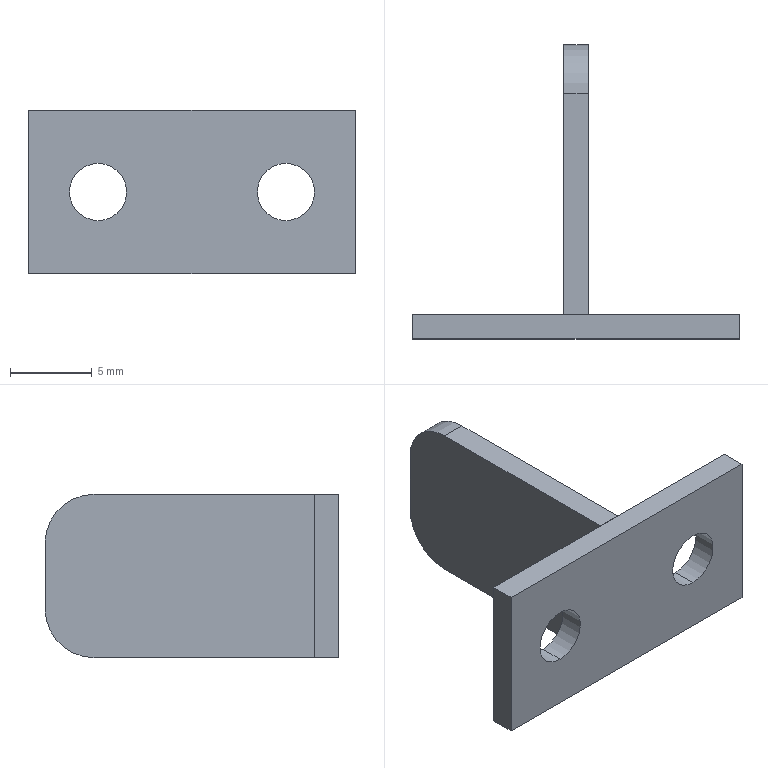Part | STEP file | Sensor detection tab | 2 solids | 18 faces | box 20 x 18 x 10 mm | volume 512.842 mm3 | plane 12 | cylinder 6 | commonest cylinder face diameters 3.5 x4 6 x2
STEP:
#1=CARTESIAN_POINT('',(0.75,13.5,-5.));
#2=VERTEX_POINT('',#1);
#3=CARTESIAN_POINT('',(0.75,0.,-5.));
#4=VERTEX_POINT('',#3);
#5=CARTESIAN_POINT('',(0.75,16.5,-5.));
#6=DIRECTION('',(0.,-1.,0.));
#7=VECTOR('',#6,1000.);
#8=LINE('',#5,#7);
#9=EDGE_CURVE('',#2,#4,#8,.T.);
#10=ORIENTED_EDGE('',*,*,#9,.F.);
#11=CARTESIAN_POINT('',(0.75,16.5,-2.));
#12=VERTEX_POINT('',#11);
#13=CARTESIAN_POINT('',(0.75,13.5,-2.));
#14=DIRECTION('',(1.,0.,0.));
#15=DIRECTION('',(0.,0.,1.));
#16=AXIS2_PLACEMENT_3D('',#13,#14,#15);
#17=CIRCLE('',#16,3.);
#18=EDGE_CURVE('',#2,#12,#17,.T.);
#19=ORIENTED_EDGE('',*,*,#18,.T.);
#20=CARTESIAN_POINT('',(0.75,16.5,2.));
#21=VERTEX_POINT('',#20);
#22=CARTESIAN_POINT('',(0.75,16.5,-5.));
#23=DIRECTION('',(0.,0.,-1.));
#24=VECTOR('',#23,1000.);
#25=LINE('',#22,#24);
#26=EDGE_CURVE('',#21,#12,#25,.T.);
#27=ORIENTED_EDGE('',*,*,#26,.F.);
#28=CARTESIAN_POINT('',(0.75,13.5,5.));
#29=VERTEX_POINT('',#28);
#30=CARTESIAN_POINT('',(0.75,13.5,2.));
#31=DIRECTION('',(1.,0.,0.));
#32=DIRECTION('',(0.,0.,1.));
#33=AXIS2_PLACEMENT_3D('',#30,#31,#32);
#34=CIRCLE('',#33,3.);
#35=EDGE_CURVE('',#21,#29,#34,.T.);
#36=ORIENTED_EDGE('',*,*,#35,.T.);
#37=CARTESIAN_POINT('',(0.75,0.,5.));
#38=VERTEX_POINT('',#37);
#39=CARTESIAN_POINT('',(0.75,16.5,5.));
#40=DIRECTION('',(0.,-1.,0.));
#41=VECTOR('',#40,1000.);
#42=LINE('',#39,#41);
#43=EDGE_CURVE('',#29,#38,#42,.T.);
#44=ORIENTED_EDGE('',*,*,#43,.T.);
#45=CARTESIAN_POINT('',(0.75,0.,-5.));
#46=DIRECTION('',(0.,0.,-1.));
#47=VECTOR('',#46,1000.);
#48=LINE('',#45,#47);
#49=EDGE_CURVE('',#38,#4,#48,.T.);
#50=ORIENTED_EDGE('',*,*,#49,.T.);
#51=EDGE_LOOP('',(#10,#19,#27,#36,#44,#50));
#52=FACE_OUTER_BOUND('',#51,.T.);
#53=CARTESIAN_POINT('',(0.75,16.5,-5.));
#54=DIRECTION('',(-1.,0.,0.));
#55=DIRECTION('',(0.,0.,1.));
#56=AXIS2_PLACEMENT_3D('',#53,#54,#55);
#57=PLANE('',#56);
#58=ADVANCED_FACE('',(#52),#57,.F.);
#59=CARTESIAN_POINT('',(-0.75,13.5,-5.));
#60=VERTEX_POINT('',#59);
#61=CARTESIAN_POINT('',(-0.75,0.,-5.));
#62=VERTEX_POINT('',#61);
#63=CARTESIAN_POINT('',(-0.75,16.5,-5.));
#64=DIRECTION('',(0.,-1.,0.));
#65=VECTOR('',#64,1000.);
#66=LINE('',#63,#65);
#67=EDGE_CURVE('',#60,#62,#66,.T.);
#68=ORIENTED_EDGE('',*,*,#67,.F.);
#69=CARTESIAN_POINT('',(0.75,13.5,-5.));
#70=DIRECTION('',(1.,0.,0.));
#71=VECTOR('',#70,1000.);
#72=LINE('',#69,#71);
#73=EDGE_CURVE('',#60,#2,#72,.T.);
#74=ORIENTED_EDGE('',*,*,#73,.T.);
#75=ORIENTED_EDGE('',*,*,#9,.T.);
#76=CARTESIAN_POINT('',(-0.75,0.,-5.));
#77=DIRECTION('',(-1.,0.,0.));
#78=VECTOR('',#77,1000.);
#79=LINE('',#76,#78);
#80=EDGE_CURVE('',#4,#62,#79,.T.);
#81=ORIENTED_EDGE('',*,*,#80,.T.);
#82=EDGE_LOOP('',(#68,#74,#75,#81));
#83=FACE_OUTER_BOUND('',#82,.T.);
#84=CARTESIAN_POINT('',(-0.75,16.5,-5.));
#85=DIRECTION('',(0.,0.,1.));
#86=DIRECTION('',(1.,0.,0.));
#87=AXIS2_PLACEMENT_3D('',#84,#85,#86);
#88=PLANE('',#87);
#89=ADVANCED_FACE('',(#83),#88,.F.);
#90=CARTESIAN_POINT('',(-0.75,16.5,-2.));
#91=VERTEX_POINT('',#90);
#92=CARTESIAN_POINT('',(-0.75,16.5,2.));
#93=VERTEX_POINT('',#92);
#94=CARTESIAN_POINT('',(-0.75,16.5,-5.));
#95=DIRECTION('',(0.,0.,1.));
#96=VECTOR('',#95,1000.);
#97=LINE('',#94,#96);
#98=EDGE_CURVE('',#91,#93,#97,.T.);
#99=ORIENTED_EDGE('',*,*,#98,.F.);
#100=CARTESIAN_POINT('',(-0.75,13.5,-2.));
#101=DIRECTION('',(-1.,0.,0.));
#102=DIRECTION('',(0.,0.,-1.));
#103=AXIS2_PLACEMENT_3D('',#100,#101,#102);
#104=CIRCLE('',#103,3.);
#105=EDGE_CURVE('',#91,#60,#104,.T.);
#106=ORIENTED_EDGE('',*,*,#105,.T.);
#107=ORIENTED_EDGE('',*,*,#67,.T.);
#108=CARTESIAN_POINT('',(-0.75,0.,5.));
#109=VERTEX_POINT('',#108);
#110=CARTESIAN_POINT('',(-0.75,0.,-5.));
#111=DIRECTION('',(0.,0.,1.));
#112=VECTOR('',#111,1000.);
#113=LINE('',#110,#112);
#114=EDGE_CURVE('',#62,#109,#113,.T.);
#115=ORIENTED_EDGE('',*,*,#114,.T.);
#116=CARTESIAN_POINT('',(-0.75,13.5,5.));
#117=VERTEX_POINT('',#116);
#118=CARTESIAN_POINT('',(-0.75,16.5,5.));
#119=DIRECTION('',(0.,-1.,0.));
#120=VECTOR('',#119,1000.);
#121=LINE('',#118,#120);
#122=EDGE_CURVE('',#117,#109,#121,.T.);
#123=ORIENTED_EDGE('',*,*,#122,.F.);
#124=CARTESIAN_POINT('',(-0.75,13.5,2.));
#125=DIRECTION('',(-1.,0.,0.));
#126=DIRECTION('',(0.,0.,-1.));
#127=AXIS2_PLACEMENT_3D('',#124,#125,#126);
#128=CIRCLE('',#127,3.);
#129=EDGE_CURVE('',#117,#93,#128,.T.);
#130=ORIENTED_EDGE('',*,*,#129,.T.);
#131=EDGE_LOOP('',(#99,#106,#107,#115,#123,#130));
#132=FACE_OUTER_BOUND('',#131,.T.);
#133=CARTESIAN_POINT('',(-0.75,16.5,-5.));
#134=DIRECTION('',(1.,0.,0.));
#135=DIRECTION('',(0.,0.,-1.));
#136=AXIS2_PLACEMENT_3D('',#133,#134,#135);
#137=PLANE('',#136);
#138=ADVANCED_FACE('',(#132),#137,.F.);
#139=ORIENTED_EDGE('',*,*,#43,.F.);
#140=CARTESIAN_POINT('',(-0.75,13.5,5.));
#141=DIRECTION('',(-1.,0.,0.));
#142=VECTOR('',#141,1000.);
#143=LINE('',#140,#142);
#144=EDGE_CURVE('',#29,#117,#143,.T.);
#145=ORIENTED_EDGE('',*,*,#144,.T.);
#146=ORIENTED_EDGE('',*,*,#122,.T.);
#147=CARTESIAN_POINT('',(-0.75,0.,5.));
#148=DIRECTION('',(1.,0.,0.));
#149=VECTOR('',#148,1000.);
#150=LINE('',#147,#149);
#151=EDGE_CURVE('',#109,#38,#150,.T.);
#152=ORIENTED_EDGE('',*,*,#151,.T.);
#153=EDGE_LOOP('',(#139,#145,#146,#152));
#154=FACE_OUTER_BOUND('',#153,.T.);
#155=CARTESIAN_POINT('',(-0.75,16.5,5.));
#156=DIRECTION('',(0.,0.,-1.));
#157=DIRECTION('',(-1.,0.,0.));
#158=AXIS2_PLACEMENT_3D('',#155,#156,#157);
#159=PLANE('',#158);
#160=ADVANCED_FACE('',(#154),#159,.F.);
#161=ORIENTED_EDGE('',*,*,#26,.T.);
#162=CARTESIAN_POINT('',(-0.75,16.5,-2.));
#163=DIRECTION('',(-1.,0.,0.));
#164=VECTOR('',#163,1000.);
#165=LINE('',#162,#164);
#166=EDGE_CURVE('',#12,#91,#165,.T.);
#167=ORIENTED_EDGE('',*,*,#166,.T.);
#168=ORIENTED_EDGE('',*,*,#98,.T.);
#169=CARTESIAN_POINT('',(0.75,16.5,2.));
#170=DIRECTION('',(1.,0.,0.));
#171=VECTOR('',#170,1000.);
#172=LINE('',#169,#171);
#173=EDGE_CURVE('',#93,#21,#172,.T.);
#174=ORIENTED_EDGE('',*,*,#173,.T.);
#175=EDGE_LOOP('',(#161,#167,#168,#174));
#176=FACE_OUTER_BOUND('',#175,.T.);
#177=CARTESIAN_POINT('',(0.,16.5,0.));
#178=DIRECTION('',(0.,1.,0.));
#179=DIRECTION('',(0.,0.,1.));
#180=AXIS2_PLACEMENT_3D('',#177,#178,#179);
#181=PLANE('',#180);
#182=ADVANCED_FACE('',(#176),#181,.T.);
#183=ORIENTED_EDGE('',*,*,#49,.F.);
#184=ORIENTED_EDGE('',*,*,#151,.F.);
#185=ORIENTED_EDGE('',*,*,#114,.F.);
#186=ORIENTED_EDGE('',*,*,#80,.F.);
#187=EDGE_LOOP('',(#183,#184,#185,#186));
#188=FACE_OUTER_BOUND('',#187,.T.);
#189=CARTESIAN_POINT('',(0.,0.,0.));
#190=DIRECTION('',(0.,1.,0.));
#191=DIRECTION('',(0.,0.,1.));
#192=AXIS2_PLACEMENT_3D('',#189,#190,#191);
#193=PLANE('',#192);
#194=ADVANCED_FACE('',(#188),#193,.F.);
#195=ORIENTED_EDGE('',*,*,#18,.F.);
#196=ORIENTED_EDGE('',*,*,#73,.F.);
#197=ORIENTED_EDGE('',*,*,#105,.F.);
#198=ORIENTED_EDGE('',*,*,#166,.F.);
#199=EDGE_LOOP('',(#195,#196,#197,#198));
#200=FACE_OUTER_BOUND('',#199,.T.);
#201=CARTESIAN_POINT('',(0.,13.5,-2.));
#202=DIRECTION('',(1.,0.,0.));
#203=DIRECTION('',(0.,0.,-1.));
#204=AXIS2_PLACEMENT_3D('',#201,#202,#203);
#205=CYLINDRICAL_SURFACE('',#204,3.);
#206=ADVANCED_FACE('',(#200),#205,.T.);
#207=ORIENTED_EDGE('',*,*,#129,.F.);
#208=ORIENTED_EDGE('',*,*,#144,.F.);
#209=ORIENTED_EDGE('',*,*,#35,.F.);
#210=ORIENTED_EDGE('',*,*,#173,.F.);
#211=EDGE_LOOP('',(#207,#208,#209,#210));
#212=FACE_OUTER_BOUND('',#211,.T.);
#213=CARTESIAN_POINT('',(0.,13.5,2.));
#214=DIRECTION('',(-1.,0.,0.));
#215=DIRECTION('',(0.,0.,1.));
#216=AXIS2_PLACEMENT_3D('',#213,#214,#215);
#217=CYLINDRICAL_SURFACE('',#216,3.);
#218=ADVANCED_FACE('',(#212),#217,.T.);
#219=CLOSED_SHELL('',(#58,#89,#138,#160,#182,#194,#206,#218));
#220=MANIFOLD_SOLID_BREP('',#219);
#221=CARTESIAN_POINT('',(-5.75,-1.5,-1.75));
#222=VERTEX_POINT('',#221);
#223=CARTESIAN_POINT('',(-5.75,-1.5,1.75));
#224=VERTEX_POINT('',#223);
#225=CARTESIAN_POINT('',(-5.75,-1.5,0.));
#226=DIRECTION('',(0.,1.,0.));
#227=DIRECTION('',(0.,0.,1.));
#228=AXIS2_PLACEMENT_3D('',#225,#226,#227);
#229=CIRCLE('',#228,1.75);
#230=EDGE_CURVE('',#222,#224,#229,.T.);
#231=ORIENTED_EDGE('',*,*,#230,.F.);
#232=CARTESIAN_POINT('',(-5.75,0.,-1.75));
#233=VERTEX_POINT('',#232);
#234=CARTESIAN_POINT('',(-5.75,0.,-1.75));
#235=DIRECTION('',(0.,1.,0.));
#236=VECTOR('',#235,1000.);
#237=LINE('',#234,#236);
#238=EDGE_CURVE('',#222,#233,#237,.T.);
#239=ORIENTED_EDGE('',*,*,#238,.T.);
#240=CARTESIAN_POINT('',(-5.75,0.,1.75));
#241=VERTEX_POINT('',#240);
#242=CARTESIAN_POINT('',(-5.75,0.,0.));
#243=DIRECTION('',(0.,1.,0.));
#244=DIRECTION('',(0.,0.,1.));
#245=AXIS2_PLACEMENT_3D('',#242,#243,#244);
#246=CIRCLE('',#245,1.75);
#247=EDGE_CURVE('',#233,#241,#246,.T.);
#248=ORIENTED_EDGE('',*,*,#247,.T.);
#249=CARTESIAN_POINT('',(-5.75,0.,1.75));
#250=DIRECTION('',(0.,1.,0.));
#251=VECTOR('',#250,1000.);
#252=LINE('',#249,#251);
#253=EDGE_CURVE('',#224,#241,#252,.T.);
#254=ORIENTED_EDGE('',*,*,#253,.F.);
#255=EDGE_LOOP('',(#231,#239,#248,#254));
#256=FACE_OUTER_BOUND('',#255,.T.);
#257=CARTESIAN_POINT('',(-5.75,0.,0.));
#258=DIRECTION('',(0.,1.,0.));
#259=DIRECTION('',(0.,0.,1.));
#260=AXIS2_PLACEMENT_3D('',#257,#258,#259);
#261=CYLINDRICAL_SURFACE('',#260,1.75);
#262=ADVANCED_FACE('',(#256),#261,.F.);
#263=CARTESIAN_POINT('',(5.75,-1.5,-1.75));
#264=VERTEX_POINT('',#263);
#265=CARTESIAN_POINT('',(5.75,-1.5,1.75));
#266=VERTEX_POINT('',#265);
#267=CARTESIAN_POINT('',(5.75,-1.5,0.));
#268=DIRECTION('',(0.,1.,0.));
#269=DIRECTION('',(0.,0.,1.));
#270=AXIS2_PLACEMENT_3D('',#267,#268,#269);
#271=CIRCLE('',#270,1.75);
#272=EDGE_CURVE('',#264,#266,#271,.T.);
#273=ORIENTED_EDGE('',*,*,#272,.F.);
#274=CARTESIAN_POINT('',(5.75,0.,-1.75));
#275=VERTEX_POINT('',#274);
#276=CARTESIAN_POINT('',(5.75,0.,-1.75));
#277=DIRECTION('',(0.,1.,0.));
#278=VECTOR('',#277,1000.);
#279=LINE('',#276,#278);
#280=EDGE_CURVE('',#264,#275,#279,.T.);
#281=ORIENTED_EDGE('',*,*,#280,.T.);
#282=CARTESIAN_POINT('',(5.75,0.,1.75));
#283=VERTEX_POINT('',#282);
#284=CARTESIAN_POINT('',(5.75,0.,0.));
#285=DIRECTION('',(0.,1.,0.));
#286=DIRECTION('',(0.,0.,1.));
#287=AXIS2_PLACEMENT_3D('',#284,#285,#286);
#288=CIRCLE('',#287,1.75);
#289=EDGE_CURVE('',#275,#283,#288,.T.);
#290=ORIENTED_EDGE('',*,*,#289,.T.);
#291=CARTESIAN_POINT('',(5.75,0.,1.75));
#292=DIRECTION('',(0.,1.,0.));
#293=VECTOR('',#292,1000.);
#294=LINE('',#291,#293);
#295=EDGE_CURVE('',#266,#283,#294,.T.);
#296=ORIENTED_EDGE('',*,*,#295,.F.);
#297=EDGE_LOOP('',(#273,#281,#290,#296));
#298=FACE_OUTER_BOUND('',#297,.T.);
#299=CARTESIAN_POINT('',(5.75,0.,0.));
#300=DIRECTION('',(0.,1.,0.));
#301=DIRECTION('',(0.,0.,1.));
#302=AXIS2_PLACEMENT_3D('',#299,#300,#301);
#303=CYLINDRICAL_SURFACE('',#302,1.75);
#304=ADVANCED_FACE('',(#298),#303,.F.);
#305=CARTESIAN_POINT('',(10.,0.,5.));
#306=VERTEX_POINT('',#305);
#307=CARTESIAN_POINT('',(10.,0.,-5.));
#308=VERTEX_POINT('',#307);
#309=CARTESIAN_POINT('',(10.,0.,-5.));
#310=DIRECTION('',(0.,0.,-1.));
#311=VECTOR('',#310,1000.);
#312=LINE('',#309,#311);
#313=EDGE_CURVE('',#306,#308,#312,.T.);
#314=ORIENTED_EDGE('',*,*,#313,.F.);
#315=CARTESIAN_POINT('',(10.,-1.5,5.));
#316=VERTEX_POINT('',#315);
#317=CARTESIAN_POINT('',(10.,-1.5,5.));
#318=DIRECTION('',(0.,1.,0.));
#319=VECTOR('',#318,1000.);
#320=LINE('',#317,#319);
#321=EDGE_CURVE('',#316,#306,#320,.T.);
#322=ORIENTED_EDGE('',*,*,#321,.F.);
#323=CARTESIAN_POINT('',(10.,-1.5,-5.));
#324=VERTEX_POINT('',#323);
#325=CARTESIAN_POINT('',(10.,-1.5,-5.));
#326=DIRECTION('',(0.,0.,-1.));
#327=VECTOR('',#326,1000.);
#328=LINE('',#325,#327);
#329=EDGE_CURVE('',#316,#324,#328,.T.);
#330=ORIENTED_EDGE('',*,*,#329,.T.);
#331=CARTESIAN_POINT('',(10.,-1.5,-5.));
#332=DIRECTION('',(0.,1.,0.));
#333=VECTOR('',#332,1000.);
#334=LINE('',#331,#333);
#335=EDGE_CURVE('',#324,#308,#334,.T.);
#336=ORIENTED_EDGE('',*,*,#335,.T.);
#337=EDGE_LOOP('',(#314,#322,#330,#336));
#338=FACE_OUTER_BOUND('',#337,.T.);
#339=CARTESIAN_POINT('',(10.,-1.5,-5.));
#340=DIRECTION('',(1.,0.,0.));
#341=DIRECTION('',(0.,0.,-1.));
#342=AXIS2_PLACEMENT_3D('',#339,#340,#341);
#343=PLANE('',#342);
#344=ADVANCED_FACE('',(#338),#343,.T.);
#345=CARTESIAN_POINT('',(-10.,0.,5.));
#346=VERTEX_POINT('',#345);
#347=CARTESIAN_POINT('',(-10.,0.,5.));
#348=DIRECTION('',(1.,0.,0.));
#349=VECTOR('',#348,1000.);
#350=LINE('',#347,#349);
#351=EDGE_CURVE('',#346,#306,#350,.T.);
#352=ORIENTED_EDGE('',*,*,#351,.F.);
#353=CARTESIAN_POINT('',(-10.,-1.5,5.));
#354=VERTEX_POINT('',#353);
#355=CARTESIAN_POINT('',(-10.,-1.5,5.));
#356=DIRECTION('',(0.,1.,0.));
#357=VECTOR('',#356,1000.);
#358=LINE('',#355,#357);
#359=EDGE_CURVE('',#354,#346,#358,.T.);
#360=ORIENTED_EDGE('',*,*,#359,.F.);
#361=CARTESIAN_POINT('',(-10.,-1.5,5.));
#362=DIRECTION('',(1.,0.,0.));
#363=VECTOR('',#362,1000.);
#364=LINE('',#361,#363);
#365=EDGE_CURVE('',#354,#316,#364,.T.);
#366=ORIENTED_EDGE('',*,*,#365,.T.);
#367=ORIENTED_EDGE('',*,*,#321,.T.);
#368=EDGE_LOOP('',(#352,#360,#366,#367));
#369=FACE_OUTER_BOUND('',#368,.T.);
#370=CARTESIAN_POINT('',(-10.,-1.5,5.));
#371=DIRECTION('',(0.,0.,1.));
#372=DIRECTION('',(1.,0.,0.));
#373=AXIS2_PLACEMENT_3D('',#370,#371,#372);
#374=PLANE('',#373);
#375=ADVANCED_FACE('',(#369),#374,.T.);
#376=CARTESIAN_POINT('',(-10.,0.,-5.));
#377=VERTEX_POINT('',#376);
#378=CARTESIAN_POINT('',(-10.,0.,-5.));
#379=DIRECTION('',(0.,0.,1.));
#380=VECTOR('',#379,1000.);
#381=LINE('',#378,#380);
#382=EDGE_CURVE('',#377,#346,#381,.T.);
#383=ORIENTED_EDGE('',*,*,#382,.F.);
#384=CARTESIAN_POINT('',(-10.,-1.5,-5.));
#385=VERTEX_POINT('',#384);
#386=CARTESIAN_POINT('',(-10.,-1.5,-5.));
#387=DIRECTION('',(0.,1.,0.));
#388=VECTOR('',#387,1000.);
#389=LINE('',#386,#388);
#390=EDGE_CURVE('',#385,#377,#389,.T.);
#391=ORIENTED_EDGE('',*,*,#390,.F.);
#392=CARTESIAN_POINT('',(-10.,-1.5,-5.));
#393=DIRECTION('',(0.,0.,1.));
#394=VECTOR('',#393,1000.);
#395=LINE('',#392,#394);
#396=EDGE_CURVE('',#385,#354,#395,.T.);
#397=ORIENTED_EDGE('',*,*,#396,.T.);
#398=ORIENTED_EDGE('',*,*,#359,.T.);
#399=EDGE_LOOP('',(#383,#391,#397,#398));
#400=FACE_OUTER_BOUND('',#399,.T.);
#401=CARTESIAN_POINT('',(-10.,-1.5,-5.));
#402=DIRECTION('',(-1.,0.,0.));
#403=DIRECTION('',(0.,0.,1.));
#404=AXIS2_PLACEMENT_3D('',#401,#402,#403);
#405=PLANE('',#404);
#406=ADVANCED_FACE('',(#400),#405,.T.);
#407=CARTESIAN_POINT('',(-10.,0.,-5.));
#408=DIRECTION('',(-1.,0.,0.));
#409=VECTOR('',#408,1000.);
#410=LINE('',#407,#409);
#411=EDGE_CURVE('',#308,#377,#410,.T.);
#412=ORIENTED_EDGE('',*,*,#411,.F.);
#413=ORIENTED_EDGE('',*,*,#335,.F.);
#414=CARTESIAN_POINT('',(-10.,-1.5,-5.));
#415=DIRECTION('',(-1.,0.,0.));
#416=VECTOR('',#415,1000.);
#417=LINE('',#414,#416);
#418=EDGE_CURVE('',#324,#385,#417,.T.);
#419=ORIENTED_EDGE('',*,*,#418,.T.);
#420=ORIENTED_EDGE('',*,*,#390,.T.);
#421=EDGE_LOOP('',(#412,#413,#419,#420));
#422=FACE_OUTER_BOUND('',#421,.T.);
#423=CARTESIAN_POINT('',(-10.,-1.5,-5.));
#424=DIRECTION('',(0.,0.,-1.));
#425=DIRECTION('',(-1.,0.,0.));
#426=AXIS2_PLACEMENT_3D('',#423,#424,#425);
#427=PLANE('',#426);
#428=ADVANCED_FACE('',(#422),#427,.T.);
#429=CARTESIAN_POINT('',(-5.75,-1.5,0.));
#430=DIRECTION('',(0.,1.,0.));
#431=DIRECTION('',(0.,0.,1.));
#432=AXIS2_PLACEMENT_3D('',#429,#430,#431);
#433=CIRCLE('',#432,1.75);
#434=EDGE_CURVE('',#224,#222,#433,.T.);
#435=ORIENTED_EDGE('',*,*,#434,.T.);
#436=ORIENTED_EDGE('',*,*,#230,.T.);
#437=EDGE_LOOP('',(#435,#436));
#438=FACE_BOUND('',#437,.T.);
#439=CARTESIAN_POINT('',(5.75,-1.5,0.));
#440=DIRECTION('',(0.,1.,0.));
#441=DIRECTION('',(0.,0.,1.));
#442=AXIS2_PLACEMENT_3D('',#439,#440,#441);
#443=CIRCLE('',#442,1.75);
#444=EDGE_CURVE('',#266,#264,#443,.T.);
#445=ORIENTED_EDGE('',*,*,#444,.T.);
#446=ORIENTED_EDGE('',*,*,#272,.T.);
#447=EDGE_LOOP('',(#445,#446));
#448=FACE_BOUND('',#447,.T.);
#449=ORIENTED_EDGE('',*,*,#329,.F.);
#450=ORIENTED_EDGE('',*,*,#365,.F.);
#451=ORIENTED_EDGE('',*,*,#396,.F.);
#452=ORIENTED_EDGE('',*,*,#418,.F.);
#453=EDGE_LOOP('',(#449,#450,#451,#452));
#454=FACE_OUTER_BOUND('',#453,.T.);
#455=CARTESIAN_POINT('',(0.,-1.5,0.));
#456=DIRECTION('',(0.,1.,0.));
#457=DIRECTION('',(0.,0.,1.));
#458=AXIS2_PLACEMENT_3D('',#455,#456,#457);
#459=PLANE('',#458);
#460=ADVANCED_FACE('',(#438,#448,#454),#459,.F.);
#461=CARTESIAN_POINT('',(-5.75,0.,0.));
#462=DIRECTION('',(0.,1.,0.));
#463=DIRECTION('',(0.,0.,1.));
#464=AXIS2_PLACEMENT_3D('',#461,#462,#463);
#465=CIRCLE('',#464,1.75);
#466=EDGE_CURVE('',#241,#233,#465,.T.);
#467=ORIENTED_EDGE('',*,*,#466,.F.);
#468=ORIENTED_EDGE('',*,*,#247,.F.);
#469=EDGE_LOOP('',(#467,#468));
#470=FACE_BOUND('',#469,.T.);
#471=CARTESIAN_POINT('',(5.75,0.,0.));
#472=DIRECTION('',(0.,1.,0.));
#473=DIRECTION('',(0.,0.,1.));
#474=AXIS2_PLACEMENT_3D('',#471,#472,#473);
#475=CIRCLE('',#474,1.75);
#476=EDGE_CURVE('',#283,#275,#475,.T.);
#477=ORIENTED_EDGE('',*,*,#476,.F.);
#478=ORIENTED_EDGE('',*,*,#289,.F.);
#479=EDGE_LOOP('',(#477,#478));
#480=FACE_BOUND('',#479,.T.);
#481=ORIENTED_EDGE('',*,*,#313,.T.);
#482=ORIENTED_EDGE('',*,*,#411,.T.);
#483=ORIENTED_EDGE('',*,*,#382,.T.);
#484=ORIENTED_EDGE('',*,*,#351,.T.);
#485=EDGE_LOOP('',(#481,#482,#483,#484));
#486=FACE_OUTER_BOUND('',#485,.T.);
#487=CARTESIAN_POINT('',(0.,0.,0.));
#488=DIRECTION('',(0.,1.,0.));
#489=DIRECTION('',(0.,0.,1.));
#490=AXIS2_PLACEMENT_3D('',#487,#488,#489);
#491=PLANE('',#490);
#492=ADVANCED_FACE('',(#470,#480,#486),#491,.T.);
#493=ORIENTED_EDGE('',*,*,#280,.F.);
#494=ORIENTED_EDGE('',*,*,#444,.F.);
#495=ORIENTED_EDGE('',*,*,#295,.T.);
#496=ORIENTED_EDGE('',*,*,#476,.T.);
#497=EDGE_LOOP('',(#493,#494,#495,#496));
#498=FACE_OUTER_BOUND('',#497,.T.);
#499=CARTESIAN_POINT('',(5.75,0.,0.));
#500=DIRECTION('',(0.,1.,0.));
#501=DIRECTION('',(0.,0.,1.));
#502=AXIS2_PLACEMENT_3D('',#499,#500,#501);
#503=CYLINDRICAL_SURFACE('',#502,1.75);
#504=ADVANCED_FACE('',(#498),#503,.F.);
#505=ORIENTED_EDGE('',*,*,#238,.F.);
#506=ORIENTED_EDGE('',*,*,#434,.F.);
#507=ORIENTED_EDGE('',*,*,#253,.T.);
#508=ORIENTED_EDGE('',*,*,#466,.T.);
#509=EDGE_LOOP('',(#505,#506,#507,#508));
#510=FACE_OUTER_BOUND('',#509,.T.);
#511=CARTESIAN_POINT('',(-5.75,0.,0.));
#512=DIRECTION('',(0.,1.,0.));
#513=DIRECTION('',(0.,0.,1.));
#514=AXIS2_PLACEMENT_3D('',#511,#512,#513);
#515=CYLINDRICAL_SURFACE('',#514,1.75);
#516=ADVANCED_FACE('',(#510),#515,.F.);
#517=CLOSED_SHELL('',(#262,#304,#344,#375,#406,#428,#460,#492,#504,#516));
#518=MANIFOLD_SOLID_BREP('',#517);
#519=CARTESIAN_POINT('',(0.,0.,0.));
#520=DIRECTION('',(0.,0.,1.));
#521=DIRECTION('',(1.,0.,0.));
#522=AXIS2_PLACEMENT_3D('',#519,#520,#521);
#523=(LENGTH_UNIT()NAMED_UNIT(*)SI_UNIT(.MILLI.,.METRE.));
#524=UNCERTAINTY_MEASURE_WITH_UNIT(LENGTH_MEASURE(0.00001),#523,'','');
#525=(NAMED_UNIT(*)PLANE_ANGLE_UNIT()SI_UNIT($,.RADIAN.));
#526=(NAMED_UNIT(*)SI_UNIT($,.STERADIAN.)SOLID_ANGLE_UNIT());
#527=(GEOMETRIC_REPRESENTATION_CONTEXT(3)GLOBAL_UNCERTAINTY_ASSIGNED_CONTEXT((#524))GLOBAL_UNIT_ASSIGNED_CONTEXT((#523,#525,#526))REPRESENTATION_CONTEXT('',''));
#528=ADVANCED_BREP_SHAPE_REPRESENTATION('',(#220,#518,#522),#527);